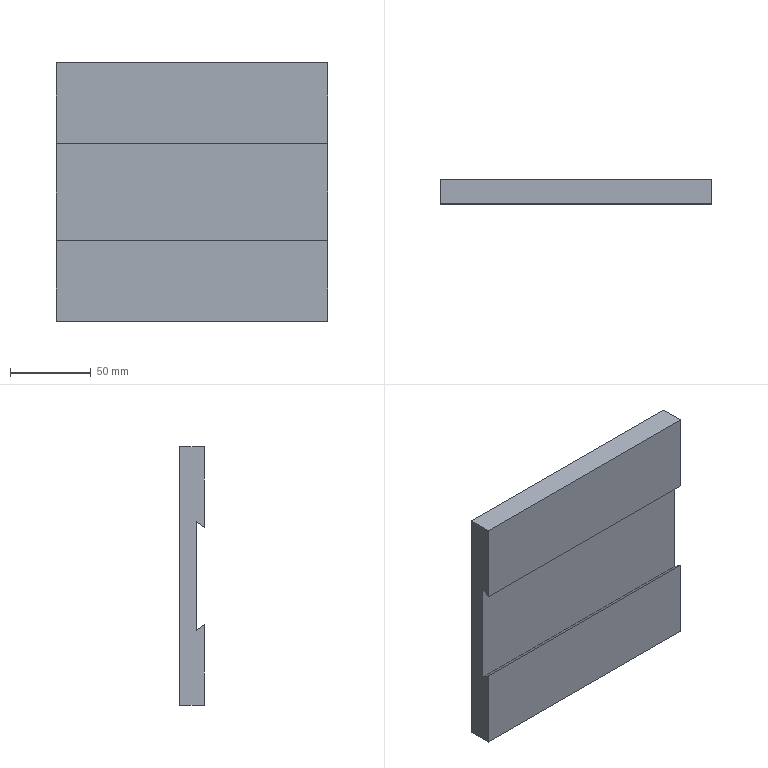Part | STEP file | 03-26 Tray support slide plate | 1 solid | 10 faces | box 168 x 15 x 160 mm | volume 349859 mm3 | plane 10
STEP:
#1=CARTESIAN_POINT('',(0.,0.,0.));
#2=DIRECTION('',(0.,0.,1.));
#3=DIRECTION('',(1.,0.,0.));
#4=AXIS2_PLACEMENT_3D('',#1,#2,#3);
#5=CARTESIAN_POINT('',(-168.,15.,80.));
#6=VERTEX_POINT('',#5);
#7=CARTESIAN_POINT('',(-168.,0.,80.));
#8=VERTEX_POINT('',#7);
#9=CARTESIAN_POINT('',(-168.,7.5,80.));
#10=DIRECTION('',(0.,-1.,0.));
#11=VECTOR('',#10,1.);
#12=LINE('',#9,#11);
#13=CARTESIAN_POINT('',(-168.,0.,80.));
#14=DIRECTION('',(0.,0.,1.));
#15=DIRECTION('',(1.,0.,0.));
#16=AXIS2_PLACEMENT_3D('',#13,#14,#15);
#17=PLANE('',#16);
#18=CARTESIAN_POINT('',(0.,7.5));
#19=DIRECTION('',(0.,-1.));
#20=VECTOR('',#19,1.);
#21=LINE('',#18,#20);
#22=(GEOMETRIC_REPRESENTATION_CONTEXT(2)PARAMETRIC_REPRESENTATION_CONTEXT()REPRESENTATION_CONTEXT('',''));
#23=DEFINITIONAL_REPRESENTATION('',(#21),#22);
#24=PCURVE('',#17,#23);
#25=CARTESIAN_POINT('',(-168.,0.,80.));
#26=DIRECTION('',(1.,0.,0.));
#27=DIRECTION('',(0.,0.,-1.));
#28=AXIS2_PLACEMENT_3D('',#25,#26,#27);
#29=PLANE('',#28);
#30=CARTESIAN_POINT('',(0.,7.5));
#31=DIRECTION('',(0.,-1.));
#32=VECTOR('',#31,1.);
#33=LINE('',#30,#32);
#34=(GEOMETRIC_REPRESENTATION_CONTEXT(2)PARAMETRIC_REPRESENTATION_CONTEXT()REPRESENTATION_CONTEXT('',''));
#35=DEFINITIONAL_REPRESENTATION('',(#33),#34);
#36=PCURVE('',#29,#35);
#37=SURFACE_CURVE('',#12,(#24,#36),.PCURVE_S1.);
#38=EDGE_CURVE('',#6,#8,#37,.T.);
#39=ORIENTED_EDGE('',*,*,#38,.T.);
#40=CARTESIAN_POINT('',(0.,0.,80.));
#41=VERTEX_POINT('',#40);
#42=CARTESIAN_POINT('',(-84.,0.,80.));
#43=DIRECTION('',(1.,0.,0.));
#44=VECTOR('',#43,1.);
#45=LINE('',#42,#44);
#46=CARTESIAN_POINT('',(84.,0.));
#47=DIRECTION('',(1.,0.));
#48=VECTOR('',#47,1.);
#49=LINE('',#46,#48);
#50=(GEOMETRIC_REPRESENTATION_CONTEXT(2)PARAMETRIC_REPRESENTATION_CONTEXT()REPRESENTATION_CONTEXT('',''));
#51=DEFINITIONAL_REPRESENTATION('',(#49),#50);
#52=PCURVE('',#17,#51);
#53=CARTESIAN_POINT('',(-168.,0.,80.));
#54=DIRECTION('',(0.,-1.,0.));
#55=DIRECTION('',(0.,0.,-1.));
#56=AXIS2_PLACEMENT_3D('',#53,#54,#55);
#57=PLANE('',#56);
#58=CARTESIAN_POINT('',(0.,84.));
#59=DIRECTION('',(0.,1.));
#60=VECTOR('',#59,1.);
#61=LINE('',#58,#60);
#62=(GEOMETRIC_REPRESENTATION_CONTEXT(2)PARAMETRIC_REPRESENTATION_CONTEXT()REPRESENTATION_CONTEXT('',''));
#63=DEFINITIONAL_REPRESENTATION('',(#61),#62);
#64=PCURVE('',#57,#63);
#65=SURFACE_CURVE('',#45,(#52,#64),.PCURVE_S1.);
#66=EDGE_CURVE('',#8,#41,#65,.T.);
#67=ORIENTED_EDGE('',*,*,#66,.T.);
#68=CARTESIAN_POINT('',(0.,15.,80.));
#69=VERTEX_POINT('',#68);
#70=CARTESIAN_POINT('',(0.,7.5,80.));
#71=DIRECTION('',(0.,1.,0.));
#72=VECTOR('',#71,1.);
#73=LINE('',#70,#72);
#74=CARTESIAN_POINT('',(168.,7.5));
#75=DIRECTION('',(0.,1.));
#76=VECTOR('',#75,1.);
#77=LINE('',#74,#76);
#78=(GEOMETRIC_REPRESENTATION_CONTEXT(2)PARAMETRIC_REPRESENTATION_CONTEXT()REPRESENTATION_CONTEXT('',''));
#79=DEFINITIONAL_REPRESENTATION('',(#77),#78);
#80=PCURVE('',#17,#79);
#81=CARTESIAN_POINT('',(0.,0.,80.));
#82=DIRECTION('',(1.,0.,0.));
#83=DIRECTION('',(0.,0.,-1.));
#84=AXIS2_PLACEMENT_3D('',#81,#82,#83);
#85=PLANE('',#84);
#86=CARTESIAN_POINT('',(0.,7.5));
#87=DIRECTION('',(0.,1.));
#88=VECTOR('',#87,1.);
#89=LINE('',#86,#88);
#90=(GEOMETRIC_REPRESENTATION_CONTEXT(2)PARAMETRIC_REPRESENTATION_CONTEXT()REPRESENTATION_CONTEXT('',''));
#91=DEFINITIONAL_REPRESENTATION('',(#89),#90);
#92=PCURVE('',#85,#91);
#93=SURFACE_CURVE('',#73,(#80,#92),.PCURVE_S1.);
#94=EDGE_CURVE('',#41,#69,#93,.T.);
#95=ORIENTED_EDGE('',*,*,#94,.T.);
#96=CARTESIAN_POINT('',(-84.,15.,80.));
#97=DIRECTION('',(-1.,0.,0.));
#98=VECTOR('',#97,1.);
#99=LINE('',#96,#98);
#100=CARTESIAN_POINT('',(84.,15.));
#101=DIRECTION('',(-1.,0.));
#102=VECTOR('',#101,1.);
#103=LINE('',#100,#102);
#104=(GEOMETRIC_REPRESENTATION_CONTEXT(2)PARAMETRIC_REPRESENTATION_CONTEXT()REPRESENTATION_CONTEXT('',''));
#105=DEFINITIONAL_REPRESENTATION('',(#103),#104);
#106=PCURVE('',#17,#105);
#107=CARTESIAN_POINT('',(-168.,15.,-80.));
#108=DIRECTION('',(0.,1.,0.));
#109=DIRECTION('',(0.,0.,1.));
#110=AXIS2_PLACEMENT_3D('',#107,#108,#109);
#111=PLANE('',#110);
#112=CARTESIAN_POINT('',(160.,84.));
#113=DIRECTION('',(0.,-1.));
#114=VECTOR('',#113,1.);
#115=LINE('',#112,#114);
#116=(GEOMETRIC_REPRESENTATION_CONTEXT(2)PARAMETRIC_REPRESENTATION_CONTEXT()REPRESENTATION_CONTEXT('',''));
#117=DEFINITIONAL_REPRESENTATION('',(#115),#116);
#118=PCURVE('',#111,#117);
#119=SURFACE_CURVE('',#99,(#106,#118),.PCURVE_S1.);
#120=EDGE_CURVE('',#69,#6,#119,.T.);
#121=ORIENTED_EDGE('',*,*,#120,.T.);
#122=EDGE_LOOP('',(#39,#67,#95,#121));
#123=FACE_BOUND('',#122,.T.);
#124=ADVANCED_FACE('',(#123),#17,.T.);
#125=CARTESIAN_POINT('',(-168.,0.,30.));
#126=VERTEX_POINT('',#125);
#127=CARTESIAN_POINT('',(-168.,0.,55.));
#128=DIRECTION('',(0.,0.,-1.));
#129=VECTOR('',#128,1.);
#130=LINE('',#127,#129);
#131=CARTESIAN_POINT('',(25.,0.));
#132=DIRECTION('',(1.,0.));
#133=VECTOR('',#132,1.);
#134=LINE('',#131,#133);
#135=(GEOMETRIC_REPRESENTATION_CONTEXT(2)PARAMETRIC_REPRESENTATION_CONTEXT()REPRESENTATION_CONTEXT('',''));
#136=DEFINITIONAL_REPRESENTATION('',(#134),#135);
#137=PCURVE('',#57,#136);
#138=CARTESIAN_POINT('',(25.,0.));
#139=DIRECTION('',(1.,0.));
#140=VECTOR('',#139,1.);
#141=LINE('',#138,#140);
#142=(GEOMETRIC_REPRESENTATION_CONTEXT(2)PARAMETRIC_REPRESENTATION_CONTEXT()REPRESENTATION_CONTEXT('',''));
#143=DEFINITIONAL_REPRESENTATION('',(#141),#142);
#144=PCURVE('',#29,#143);
#145=SURFACE_CURVE('',#130,(#137,#144),.PCURVE_S1.);
#146=EDGE_CURVE('',#8,#126,#145,.T.);
#147=ORIENTED_EDGE('',*,*,#146,.T.);
#148=CARTESIAN_POINT('',(0.,0.,30.));
#149=VERTEX_POINT('',#148);
#150=CARTESIAN_POINT('',(-84.,0.,30.));
#151=DIRECTION('',(1.,0.,0.));
#152=VECTOR('',#151,1.);
#153=LINE('',#150,#152);
#154=CARTESIAN_POINT('',(50.,84.));
#155=DIRECTION('',(0.,1.));
#156=VECTOR('',#155,1.);
#157=LINE('',#154,#156);
#158=(GEOMETRIC_REPRESENTATION_CONTEXT(2)PARAMETRIC_REPRESENTATION_CONTEXT()REPRESENTATION_CONTEXT('',''));
#159=DEFINITIONAL_REPRESENTATION('',(#157),#158);
#160=PCURVE('',#57,#159);
#161=CARTESIAN_POINT('',(-168.,0.,30.));
#162=DIRECTION('',(0.,0.5736,-0.8192));
#163=DIRECTION('',(0.,0.8192,0.5736));
#164=AXIS2_PLACEMENT_3D('',#161,#162,#163);
#165=PLANE('',#164);
#166=CARTESIAN_POINT('',(0.,84.));
#167=DIRECTION('',(0.,1.));
#168=VECTOR('',#167,1.);
#169=LINE('',#166,#168);
#170=(GEOMETRIC_REPRESENTATION_CONTEXT(2)PARAMETRIC_REPRESENTATION_CONTEXT()REPRESENTATION_CONTEXT('',''));
#171=DEFINITIONAL_REPRESENTATION('',(#169),#170);
#172=PCURVE('',#165,#171);
#173=SURFACE_CURVE('',#153,(#160,#172),.PCURVE_S1.);
#174=EDGE_CURVE('',#126,#149,#173,.T.);
#175=ORIENTED_EDGE('',*,*,#174,.T.);
#176=CARTESIAN_POINT('',(0.,0.,55.));
#177=DIRECTION('',(0.,0.,1.));
#178=VECTOR('',#177,1.);
#179=LINE('',#176,#178);
#180=CARTESIAN_POINT('',(25.,168.));
#181=DIRECTION('',(-1.,0.));
#182=VECTOR('',#181,1.);
#183=LINE('',#180,#182);
#184=(GEOMETRIC_REPRESENTATION_CONTEXT(2)PARAMETRIC_REPRESENTATION_CONTEXT()REPRESENTATION_CONTEXT('',''));
#185=DEFINITIONAL_REPRESENTATION('',(#183),#184);
#186=PCURVE('',#57,#185);
#187=CARTESIAN_POINT('',(25.,0.));
#188=DIRECTION('',(-1.,0.));
#189=VECTOR('',#188,1.);
#190=LINE('',#187,#189);
#191=(GEOMETRIC_REPRESENTATION_CONTEXT(2)PARAMETRIC_REPRESENTATION_CONTEXT()REPRESENTATION_CONTEXT('',''));
#192=DEFINITIONAL_REPRESENTATION('',(#190),#191);
#193=PCURVE('',#85,#192);
#194=SURFACE_CURVE('',#179,(#186,#193),.PCURVE_S1.);
#195=EDGE_CURVE('',#149,#41,#194,.T.);
#196=ORIENTED_EDGE('',*,*,#195,.T.);
#197=ORIENTED_EDGE('',*,*,#66,.F.);
#198=EDGE_LOOP('',(#147,#175,#196,#197));
#199=FACE_BOUND('',#198,.T.);
#200=ADVANCED_FACE('',(#199),#57,.T.);
#201=CARTESIAN_POINT('',(-168.,15.,-80.));
#202=VERTEX_POINT('',#201);
#203=CARTESIAN_POINT('',(-168.,15.,0.));
#204=DIRECTION('',(0.,0.,1.));
#205=VECTOR('',#204,1.);
#206=LINE('',#203,#205);
#207=CARTESIAN_POINT('',(80.,15.));
#208=DIRECTION('',(-1.,0.));
#209=VECTOR('',#208,1.);
#210=LINE('',#207,#209);
#211=(GEOMETRIC_REPRESENTATION_CONTEXT(2)PARAMETRIC_REPRESENTATION_CONTEXT()REPRESENTATION_CONTEXT('',''));
#212=DEFINITIONAL_REPRESENTATION('',(#210),#211);
#213=PCURVE('',#29,#212);
#214=CARTESIAN_POINT('',(80.,0.));
#215=DIRECTION('',(1.,0.));
#216=VECTOR('',#215,1.);
#217=LINE('',#214,#216);
#218=(GEOMETRIC_REPRESENTATION_CONTEXT(2)PARAMETRIC_REPRESENTATION_CONTEXT()REPRESENTATION_CONTEXT('',''));
#219=DEFINITIONAL_REPRESENTATION('',(#217),#218);
#220=PCURVE('',#111,#219);
#221=SURFACE_CURVE('',#206,(#213,#220),.PCURVE_S1.);
#222=EDGE_CURVE('',#202,#6,#221,.T.);
#223=ORIENTED_EDGE('',*,*,#222,.F.);
#224=CARTESIAN_POINT('',(-168.,0.,-80.));
#225=VERTEX_POINT('',#224);
#226=CARTESIAN_POINT('',(-168.,7.5,-80.));
#227=DIRECTION('',(0.,1.,0.));
#228=VECTOR('',#227,1.);
#229=LINE('',#226,#228);
#230=CARTESIAN_POINT('',(160.,7.5));
#231=DIRECTION('',(0.,1.));
#232=VECTOR('',#231,1.);
#233=LINE('',#230,#232);
#234=(GEOMETRIC_REPRESENTATION_CONTEXT(2)PARAMETRIC_REPRESENTATION_CONTEXT()REPRESENTATION_CONTEXT('',''));
#235=DEFINITIONAL_REPRESENTATION('',(#233),#234);
#236=PCURVE('',#29,#235);
#237=CARTESIAN_POINT('',(0.,0.,-80.));
#238=DIRECTION('',(0.,0.,-1.));
#239=DIRECTION('',(-1.,0.,0.));
#240=AXIS2_PLACEMENT_3D('',#237,#238,#239);
#241=PLANE('',#240);
#242=CARTESIAN_POINT('',(168.,7.5));
#243=DIRECTION('',(0.,1.));
#244=VECTOR('',#243,1.);
#245=LINE('',#242,#244);
#246=(GEOMETRIC_REPRESENTATION_CONTEXT(2)PARAMETRIC_REPRESENTATION_CONTEXT()REPRESENTATION_CONTEXT('',''));
#247=DEFINITIONAL_REPRESENTATION('',(#245),#246);
#248=PCURVE('',#241,#247);
#249=SURFACE_CURVE('',#229,(#236,#248),.PCURVE_S1.);
#250=EDGE_CURVE('',#225,#202,#249,.T.);
#251=ORIENTED_EDGE('',*,*,#250,.F.);
#252=CARTESIAN_POINT('',(-168.,0.,-30.));
#253=VERTEX_POINT('',#252);
#254=CARTESIAN_POINT('',(-168.,0.,0.));
#255=DIRECTION('',(0.,0.,-1.));
#256=VECTOR('',#255,1.);
#257=LINE('',#254,#256);
#258=CARTESIAN_POINT('',(80.,0.));
#259=DIRECTION('',(1.,0.));
#260=VECTOR('',#259,1.);
#261=LINE('',#258,#260);
#262=(GEOMETRIC_REPRESENTATION_CONTEXT(2)PARAMETRIC_REPRESENTATION_CONTEXT()REPRESENTATION_CONTEXT('',''));
#263=DEFINITIONAL_REPRESENTATION('',(#261),#262);
#264=PCURVE('',#29,#263);
#265=CARTESIAN_POINT('',(-168.,0.,-30.));
#266=DIRECTION('',(0.,-1.,0.));
#267=DIRECTION('',(0.,0.,-1.));
#268=AXIS2_PLACEMENT_3D('',#265,#266,#267);
#269=PLANE('',#268);
#270=CARTESIAN_POINT('',(-30.,0.));
#271=DIRECTION('',(1.,0.));
#272=VECTOR('',#271,1.);
#273=LINE('',#270,#272);
#274=(GEOMETRIC_REPRESENTATION_CONTEXT(2)PARAMETRIC_REPRESENTATION_CONTEXT()REPRESENTATION_CONTEXT('',''));
#275=DEFINITIONAL_REPRESENTATION('',(#273),#274);
#276=PCURVE('',#269,#275);
#277=SURFACE_CURVE('',#257,(#264,#276),.PCURVE_S1.);
#278=EDGE_CURVE('',#253,#225,#277,.T.);
#279=ORIENTED_EDGE('',*,*,#278,.F.);
#280=CARTESIAN_POINT('',(-168.,5.,-33.501));
#281=VERTEX_POINT('',#280);
#282=CARTESIAN_POINT('',(-168.,5.,-33.501));
#283=DIRECTION('',(0.,-0.8192,0.5736));
#284=VECTOR('',#283,1.);
#285=LINE('',#282,#284);
#286=CARTESIAN_POINT('',(113.501,5.));
#287=DIRECTION('',(-0.5736,-0.8192));
#288=VECTOR('',#287,1.);
#289=LINE('',#286,#288);
#290=(GEOMETRIC_REPRESENTATION_CONTEXT(2)PARAMETRIC_REPRESENTATION_CONTEXT()REPRESENTATION_CONTEXT('',''));
#291=DEFINITIONAL_REPRESENTATION('',(#289),#290);
#292=PCURVE('',#29,#291);
#293=CARTESIAN_POINT('',(-168.,5.,-33.501));
#294=DIRECTION('',(0.,0.5736,0.8192));
#295=DIRECTION('',(0.,-0.8192,0.5736));
#296=AXIS2_PLACEMENT_3D('',#293,#294,#295);
#297=PLANE('',#296);
#298=CARTESIAN_POINT('',(0.,0.));
#299=DIRECTION('',(1.,0.));
#300=VECTOR('',#299,1.);
#301=LINE('',#298,#300);
#302=(GEOMETRIC_REPRESENTATION_CONTEXT(2)PARAMETRIC_REPRESENTATION_CONTEXT()REPRESENTATION_CONTEXT('',''));
#303=DEFINITIONAL_REPRESENTATION('',(#301),#302);
#304=PCURVE('',#297,#303);
#305=SURFACE_CURVE('',#285,(#292,#304),.PCURVE_S1.);
#306=EDGE_CURVE('',#281,#253,#305,.T.);
#307=ORIENTED_EDGE('',*,*,#306,.F.);
#308=CARTESIAN_POINT('',(-168.,5.,33.501));
#309=VERTEX_POINT('',#308);
#310=CARTESIAN_POINT('',(-168.,5.,0.));
#311=DIRECTION('',(0.,0.,-1.));
#312=VECTOR('',#311,1.);
#313=LINE('',#310,#312);
#314=CARTESIAN_POINT('',(80.,5.));
#315=DIRECTION('',(1.,0.));
#316=VECTOR('',#315,1.);
#317=LINE('',#314,#316);
#318=(GEOMETRIC_REPRESENTATION_CONTEXT(2)PARAMETRIC_REPRESENTATION_CONTEXT()REPRESENTATION_CONTEXT('',''));
#319=DEFINITIONAL_REPRESENTATION('',(#317),#318);
#320=PCURVE('',#29,#319);
#321=CARTESIAN_POINT('',(-168.,5.,33.501));
#322=DIRECTION('',(0.,-1.,0.));
#323=DIRECTION('',(0.,0.,-1.));
#324=AXIS2_PLACEMENT_3D('',#321,#322,#323);
#325=PLANE('',#324);
#326=CARTESIAN_POINT('',(33.501,0.));
#327=DIRECTION('',(1.,0.));
#328=VECTOR('',#327,1.);
#329=LINE('',#326,#328);
#330=(GEOMETRIC_REPRESENTATION_CONTEXT(2)PARAMETRIC_REPRESENTATION_CONTEXT()REPRESENTATION_CONTEXT('',''));
#331=DEFINITIONAL_REPRESENTATION('',(#329),#330);
#332=PCURVE('',#325,#331);
#333=SURFACE_CURVE('',#313,(#320,#332),.PCURVE_S1.);
#334=EDGE_CURVE('',#309,#281,#333,.T.);
#335=ORIENTED_EDGE('',*,*,#334,.F.);
#336=CARTESIAN_POINT('',(-168.,0.,30.));
#337=DIRECTION('',(0.,0.8192,0.5736));
#338=VECTOR('',#337,1.);
#339=LINE('',#336,#338);
#340=CARTESIAN_POINT('',(50.,0.));
#341=DIRECTION('',(-0.5736,0.8192));
#342=VECTOR('',#341,1.);
#343=LINE('',#340,#342);
#344=(GEOMETRIC_REPRESENTATION_CONTEXT(2)PARAMETRIC_REPRESENTATION_CONTEXT()REPRESENTATION_CONTEXT('',''));
#345=DEFINITIONAL_REPRESENTATION('',(#343),#344);
#346=PCURVE('',#29,#345);
#347=CARTESIAN_POINT('',(0.,0.));
#348=DIRECTION('',(1.,0.));
#349=VECTOR('',#348,1.);
#350=LINE('',#347,#349);
#351=(GEOMETRIC_REPRESENTATION_CONTEXT(2)PARAMETRIC_REPRESENTATION_CONTEXT()REPRESENTATION_CONTEXT('',''));
#352=DEFINITIONAL_REPRESENTATION('',(#350),#351);
#353=PCURVE('',#165,#352);
#354=SURFACE_CURVE('',#339,(#346,#353),.PCURVE_S1.);
#355=EDGE_CURVE('',#126,#309,#354,.T.);
#356=ORIENTED_EDGE('',*,*,#355,.F.);
#357=ORIENTED_EDGE('',*,*,#146,.F.);
#358=ORIENTED_EDGE('',*,*,#38,.F.);
#359=EDGE_LOOP('',(#223,#251,#279,#307,#335,#356,#357,#358));
#360=FACE_BOUND('',#359,.T.);
#361=ADVANCED_FACE('',(#360),#29,.F.);
#362=ORIENTED_EDGE('',*,*,#222,.T.);
#363=ORIENTED_EDGE('',*,*,#120,.F.);
#364=CARTESIAN_POINT('',(0.,15.,-80.));
#365=VERTEX_POINT('',#364);
#366=CARTESIAN_POINT('',(0.,15.,0.));
#367=DIRECTION('',(0.,0.,-1.));
#368=VECTOR('',#367,1.);
#369=LINE('',#366,#368);
#370=CARTESIAN_POINT('',(80.,168.));
#371=DIRECTION('',(-1.,0.));
#372=VECTOR('',#371,1.);
#373=LINE('',#370,#372);
#374=(GEOMETRIC_REPRESENTATION_CONTEXT(2)PARAMETRIC_REPRESENTATION_CONTEXT()REPRESENTATION_CONTEXT('',''));
#375=DEFINITIONAL_REPRESENTATION('',(#373),#374);
#376=PCURVE('',#111,#375);
#377=CARTESIAN_POINT('',(80.,15.));
#378=DIRECTION('',(1.,0.));
#379=VECTOR('',#378,1.);
#380=LINE('',#377,#379);
#381=(GEOMETRIC_REPRESENTATION_CONTEXT(2)PARAMETRIC_REPRESENTATION_CONTEXT()REPRESENTATION_CONTEXT('',''));
#382=DEFINITIONAL_REPRESENTATION('',(#380),#381);
#383=PCURVE('',#85,#382);
#384=SURFACE_CURVE('',#369,(#376,#383),.PCURVE_S1.);
#385=EDGE_CURVE('',#69,#365,#384,.T.);
#386=ORIENTED_EDGE('',*,*,#385,.T.);
#387=CARTESIAN_POINT('',(-84.,15.,-80.));
#388=DIRECTION('',(-1.,0.,0.));
#389=VECTOR('',#388,1.);
#390=LINE('',#387,#389);
#391=CARTESIAN_POINT('',(0.,84.));
#392=DIRECTION('',(0.,-1.));
#393=VECTOR('',#392,1.);
#394=LINE('',#391,#393);
#395=(GEOMETRIC_REPRESENTATION_CONTEXT(2)PARAMETRIC_REPRESENTATION_CONTEXT()REPRESENTATION_CONTEXT('',''));
#396=DEFINITIONAL_REPRESENTATION('',(#394),#395);
#397=PCURVE('',#111,#396);
#398=CARTESIAN_POINT('',(84.,15.));
#399=DIRECTION('',(1.,0.));
#400=VECTOR('',#399,1.);
#401=LINE('',#398,#400);
#402=(GEOMETRIC_REPRESENTATION_CONTEXT(2)PARAMETRIC_REPRESENTATION_CONTEXT()REPRESENTATION_CONTEXT('',''));
#403=DEFINITIONAL_REPRESENTATION('',(#401),#402);
#404=PCURVE('',#241,#403);
#405=SURFACE_CURVE('',#390,(#397,#404),.PCURVE_S1.);
#406=EDGE_CURVE('',#365,#202,#405,.T.);
#407=ORIENTED_EDGE('',*,*,#406,.T.);
#408=EDGE_LOOP('',(#362,#363,#386,#407));
#409=FACE_BOUND('',#408,.T.);
#410=ADVANCED_FACE('',(#409),#111,.T.);
#411=CARTESIAN_POINT('',(0.,0.,-80.));
#412=VERTEX_POINT('',#411);
#413=CARTESIAN_POINT('',(0.,7.5,-80.));
#414=DIRECTION('',(0.,1.,0.));
#415=VECTOR('',#414,1.);
#416=LINE('',#413,#415);
#417=CARTESIAN_POINT('',(160.,7.5));
#418=DIRECTION('',(0.,1.));
#419=VECTOR('',#418,1.);
#420=LINE('',#417,#419);
#421=(GEOMETRIC_REPRESENTATION_CONTEXT(2)PARAMETRIC_REPRESENTATION_CONTEXT()REPRESENTATION_CONTEXT('',''));
#422=DEFINITIONAL_REPRESENTATION('',(#420),#421);
#423=PCURVE('',#85,#422);
#424=CARTESIAN_POINT('',(0.,7.5));
#425=DIRECTION('',(0.,1.));
#426=VECTOR('',#425,1.);
#427=LINE('',#424,#426);
#428=(GEOMETRIC_REPRESENTATION_CONTEXT(2)PARAMETRIC_REPRESENTATION_CONTEXT()REPRESENTATION_CONTEXT('',''));
#429=DEFINITIONAL_REPRESENTATION('',(#427),#428);
#430=PCURVE('',#241,#429);
#431=SURFACE_CURVE('',#416,(#423,#430),.PCURVE_S1.);
#432=EDGE_CURVE('',#412,#365,#431,.T.);
#433=ORIENTED_EDGE('',*,*,#432,.T.);
#434=ORIENTED_EDGE('',*,*,#385,.F.);
#435=ORIENTED_EDGE('',*,*,#94,.F.);
#436=ORIENTED_EDGE('',*,*,#195,.F.);
#437=CARTESIAN_POINT('',(0.,5.,33.501));
#438=VERTEX_POINT('',#437);
#439=CARTESIAN_POINT('',(0.,0.,30.));
#440=DIRECTION('',(0.,0.8192,0.5736));
#441=VECTOR('',#440,1.);
#442=LINE('',#439,#441);
#443=CARTESIAN_POINT('',(50.,0.));
#444=DIRECTION('',(-0.5736,0.8192));
#445=VECTOR('',#444,1.);
#446=LINE('',#443,#445);
#447=(GEOMETRIC_REPRESENTATION_CONTEXT(2)PARAMETRIC_REPRESENTATION_CONTEXT()REPRESENTATION_CONTEXT('',''));
#448=DEFINITIONAL_REPRESENTATION('',(#446),#447);
#449=PCURVE('',#85,#448);
#450=CARTESIAN_POINT('',(0.,168.));
#451=DIRECTION('',(1.,0.));
#452=VECTOR('',#451,1.);
#453=LINE('',#450,#452);
#454=(GEOMETRIC_REPRESENTATION_CONTEXT(2)PARAMETRIC_REPRESENTATION_CONTEXT()REPRESENTATION_CONTEXT('',''));
#455=DEFINITIONAL_REPRESENTATION('',(#453),#454);
#456=PCURVE('',#165,#455);
#457=SURFACE_CURVE('',#442,(#449,#456),.PCURVE_S1.);
#458=EDGE_CURVE('',#149,#438,#457,.T.);
#459=ORIENTED_EDGE('',*,*,#458,.T.);
#460=CARTESIAN_POINT('',(0.,5.,-33.501));
#461=VERTEX_POINT('',#460);
#462=CARTESIAN_POINT('',(0.,5.,0.));
#463=DIRECTION('',(0.,0.,-1.));
#464=VECTOR('',#463,1.);
#465=LINE('',#462,#464);
#466=CARTESIAN_POINT('',(80.,5.));
#467=DIRECTION('',(1.,0.));
#468=VECTOR('',#467,1.);
#469=LINE('',#466,#468);
#470=(GEOMETRIC_REPRESENTATION_CONTEXT(2)PARAMETRIC_REPRESENTATION_CONTEXT()REPRESENTATION_CONTEXT('',''));
#471=DEFINITIONAL_REPRESENTATION('',(#469),#470);
#472=PCURVE('',#85,#471);
#473=CARTESIAN_POINT('',(33.501,168.));
#474=DIRECTION('',(1.,0.));
#475=VECTOR('',#474,1.);
#476=LINE('',#473,#475);
#477=(GEOMETRIC_REPRESENTATION_CONTEXT(2)PARAMETRIC_REPRESENTATION_CONTEXT()REPRESENTATION_CONTEXT('',''));
#478=DEFINITIONAL_REPRESENTATION('',(#476),#477);
#479=PCURVE('',#325,#478);
#480=SURFACE_CURVE('',#465,(#472,#479),.PCURVE_S1.);
#481=EDGE_CURVE('',#438,#461,#480,.T.);
#482=ORIENTED_EDGE('',*,*,#481,.T.);
#483=CARTESIAN_POINT('',(0.,0.,-30.));
#484=VERTEX_POINT('',#483);
#485=CARTESIAN_POINT('',(0.,5.,-33.501));
#486=DIRECTION('',(0.,-0.8192,0.5736));
#487=VECTOR('',#486,1.);
#488=LINE('',#485,#487);
#489=CARTESIAN_POINT('',(113.501,5.));
#490=DIRECTION('',(-0.5736,-0.8192));
#491=VECTOR('',#490,1.);
#492=LINE('',#489,#491);
#493=(GEOMETRIC_REPRESENTATION_CONTEXT(2)PARAMETRIC_REPRESENTATION_CONTEXT()REPRESENTATION_CONTEXT('',''));
#494=DEFINITIONAL_REPRESENTATION('',(#492),#493);
#495=PCURVE('',#85,#494);
#496=CARTESIAN_POINT('',(-0.000000035,168.));
#497=DIRECTION('',(1.,0.));
#498=VECTOR('',#497,1.);
#499=LINE('',#496,#498);
#500=(GEOMETRIC_REPRESENTATION_CONTEXT(2)PARAMETRIC_REPRESENTATION_CONTEXT()REPRESENTATION_CONTEXT('',''));
#501=DEFINITIONAL_REPRESENTATION('',(#499),#500);
#502=PCURVE('',#297,#501);
#503=SURFACE_CURVE('',#488,(#495,#502),.PCURVE_S1.);
#504=EDGE_CURVE('',#461,#484,#503,.T.);
#505=ORIENTED_EDGE('',*,*,#504,.T.);
#506=CARTESIAN_POINT('',(0.,0.,0.));
#507=DIRECTION('',(0.,0.,-1.));
#508=VECTOR('',#507,1.);
#509=LINE('',#506,#508);
#510=CARTESIAN_POINT('',(80.,0.));
#511=DIRECTION('',(1.,0.));
#512=VECTOR('',#511,1.);
#513=LINE('',#510,#512);
#514=(GEOMETRIC_REPRESENTATION_CONTEXT(2)PARAMETRIC_REPRESENTATION_CONTEXT()REPRESENTATION_CONTEXT('',''));
#515=DEFINITIONAL_REPRESENTATION('',(#513),#514);
#516=PCURVE('',#85,#515);
#517=CARTESIAN_POINT('',(-30.,168.));
#518=DIRECTION('',(1.,0.));
#519=VECTOR('',#518,1.);
#520=LINE('',#517,#519);
#521=(GEOMETRIC_REPRESENTATION_CONTEXT(2)PARAMETRIC_REPRESENTATION_CONTEXT()REPRESENTATION_CONTEXT('',''));
#522=DEFINITIONAL_REPRESENTATION('',(#520),#521);
#523=PCURVE('',#269,#522);
#524=SURFACE_CURVE('',#509,(#516,#523),.PCURVE_S1.);
#525=EDGE_CURVE('',#484,#412,#524,.T.);
#526=ORIENTED_EDGE('',*,*,#525,.T.);
#527=EDGE_LOOP('',(#433,#434,#435,#436,#459,#482,#505,#526));
#528=FACE_BOUND('',#527,.T.);
#529=ADVANCED_FACE('',(#528),#85,.T.);
#530=ORIENTED_EDGE('',*,*,#355,.T.);
#531=CARTESIAN_POINT('',(-84.,5.,33.501));
#532=DIRECTION('',(1.,0.,0.));
#533=VECTOR('',#532,1.);
#534=LINE('',#531,#533);
#535=CARTESIAN_POINT('',(6.104,84.));
#536=DIRECTION('',(0.,1.));
#537=VECTOR('',#536,1.);
#538=LINE('',#535,#537);
#539=(GEOMETRIC_REPRESENTATION_CONTEXT(2)PARAMETRIC_REPRESENTATION_CONTEXT()REPRESENTATION_CONTEXT('',''));
#540=DEFINITIONAL_REPRESENTATION('',(#538),#539);
#541=PCURVE('',#165,#540);
#542=CARTESIAN_POINT('',(0.,84.));
#543=DIRECTION('',(0.,1.));
#544=VECTOR('',#543,1.);
#545=LINE('',#542,#544);
#546=(GEOMETRIC_REPRESENTATION_CONTEXT(2)PARAMETRIC_REPRESENTATION_CONTEXT()REPRESENTATION_CONTEXT('',''));
#547=DEFINITIONAL_REPRESENTATION('',(#545),#546);
#548=PCURVE('',#325,#547);
#549=SURFACE_CURVE('',#534,(#541,#548),.PCURVE_S1.);
#550=EDGE_CURVE('',#309,#438,#549,.T.);
#551=ORIENTED_EDGE('',*,*,#550,.T.);
#552=ORIENTED_EDGE('',*,*,#458,.F.);
#553=ORIENTED_EDGE('',*,*,#174,.F.);
#554=EDGE_LOOP('',(#530,#551,#552,#553));
#555=FACE_BOUND('',#554,.T.);
#556=ADVANCED_FACE('',(#555),#165,.T.);
#557=ORIENTED_EDGE('',*,*,#250,.T.);
#558=ORIENTED_EDGE('',*,*,#406,.F.);
#559=ORIENTED_EDGE('',*,*,#432,.F.);
#560=CARTESIAN_POINT('',(-84.,0.,-80.));
#561=DIRECTION('',(-1.,0.,0.));
#562=VECTOR('',#561,1.);
#563=LINE('',#560,#562);
#564=CARTESIAN_POINT('',(84.,0.));
#565=DIRECTION('',(1.,0.));
#566=VECTOR('',#565,1.);
#567=LINE('',#564,#566);
#568=(GEOMETRIC_REPRESENTATION_CONTEXT(2)PARAMETRIC_REPRESENTATION_CONTEXT()REPRESENTATION_CONTEXT('',''));
#569=DEFINITIONAL_REPRESENTATION('',(#567),#568);
#570=PCURVE('',#241,#569);
#571=CARTESIAN_POINT('',(50.,84.));
#572=DIRECTION('',(0.,-1.));
#573=VECTOR('',#572,1.);
#574=LINE('',#571,#573);
#575=(GEOMETRIC_REPRESENTATION_CONTEXT(2)PARAMETRIC_REPRESENTATION_CONTEXT()REPRESENTATION_CONTEXT('',''));
#576=DEFINITIONAL_REPRESENTATION('',(#574),#575);
#577=PCURVE('',#269,#576);
#578=SURFACE_CURVE('',#563,(#570,#577),.PCURVE_S1.);
#579=EDGE_CURVE('',#412,#225,#578,.T.);
#580=ORIENTED_EDGE('',*,*,#579,.T.);
#581=EDGE_LOOP('',(#557,#558,#559,#580));
#582=FACE_BOUND('',#581,.T.);
#583=ADVANCED_FACE('',(#582),#241,.T.);
#584=ORIENTED_EDGE('',*,*,#278,.T.);
#585=ORIENTED_EDGE('',*,*,#579,.F.);
#586=ORIENTED_EDGE('',*,*,#525,.F.);
#587=CARTESIAN_POINT('',(-84.,0.,-30.));
#588=DIRECTION('',(-1.,0.,0.));
#589=VECTOR('',#588,1.);
#590=LINE('',#587,#589);
#591=CARTESIAN_POINT('',(0.,84.));
#592=DIRECTION('',(0.,-1.));
#593=VECTOR('',#592,1.);
#594=LINE('',#591,#593);
#595=(GEOMETRIC_REPRESENTATION_CONTEXT(2)PARAMETRIC_REPRESENTATION_CONTEXT()REPRESENTATION_CONTEXT('',''));
#596=DEFINITIONAL_REPRESENTATION('',(#594),#595);
#597=PCURVE('',#269,#596);
#598=CARTESIAN_POINT('',(6.104,84.));
#599=DIRECTION('',(0.,-1.));
#600=VECTOR('',#599,1.);
#601=LINE('',#598,#600);
#602=(GEOMETRIC_REPRESENTATION_CONTEXT(2)PARAMETRIC_REPRESENTATION_CONTEXT()REPRESENTATION_CONTEXT('',''));
#603=DEFINITIONAL_REPRESENTATION('',(#601),#602);
#604=PCURVE('',#297,#603);
#605=SURFACE_CURVE('',#590,(#597,#604),.PCURVE_S1.);
#606=EDGE_CURVE('',#484,#253,#605,.T.);
#607=ORIENTED_EDGE('',*,*,#606,.T.);
#608=EDGE_LOOP('',(#584,#585,#586,#607));
#609=FACE_BOUND('',#608,.T.);
#610=ADVANCED_FACE('',(#609),#269,.T.);
#611=ORIENTED_EDGE('',*,*,#306,.T.);
#612=ORIENTED_EDGE('',*,*,#606,.F.);
#613=ORIENTED_EDGE('',*,*,#504,.F.);
#614=CARTESIAN_POINT('',(-84.,5.,-33.501));
#615=DIRECTION('',(-1.,0.,0.));
#616=VECTOR('',#615,1.);
#617=LINE('',#614,#616);
#618=CARTESIAN_POINT('',(0.,84.));
#619=DIRECTION('',(0.,-1.));
#620=VECTOR('',#619,1.);
#621=LINE('',#618,#620);
#622=(GEOMETRIC_REPRESENTATION_CONTEXT(2)PARAMETRIC_REPRESENTATION_CONTEXT()REPRESENTATION_CONTEXT('',''));
#623=DEFINITIONAL_REPRESENTATION('',(#621),#622);
#624=PCURVE('',#297,#623);
#625=CARTESIAN_POINT('',(67.002,84.));
#626=DIRECTION('',(0.,-1.));
#627=VECTOR('',#626,1.);
#628=LINE('',#625,#627);
#629=(GEOMETRIC_REPRESENTATION_CONTEXT(2)PARAMETRIC_REPRESENTATION_CONTEXT()REPRESENTATION_CONTEXT('',''));
#630=DEFINITIONAL_REPRESENTATION('',(#628),#629);
#631=PCURVE('',#325,#630);
#632=SURFACE_CURVE('',#617,(#624,#631),.PCURVE_S1.);
#633=EDGE_CURVE('',#461,#281,#632,.T.);
#634=ORIENTED_EDGE('',*,*,#633,.T.);
#635=EDGE_LOOP('',(#611,#612,#613,#634));
#636=FACE_BOUND('',#635,.T.);
#637=ADVANCED_FACE('',(#636),#297,.T.);
#638=ORIENTED_EDGE('',*,*,#334,.T.);
#639=ORIENTED_EDGE('',*,*,#633,.F.);
#640=ORIENTED_EDGE('',*,*,#481,.F.);
#641=ORIENTED_EDGE('',*,*,#550,.F.);
#642=EDGE_LOOP('',(#638,#639,#640,#641));
#643=FACE_BOUND('',#642,.T.);
#644=ADVANCED_FACE('',(#643),#325,.T.);
#645=CLOSED_SHELL('',(#124,#200,#361,#410,#529,#556,#583,#610,#637,#644));
#646=MANIFOLD_SOLID_BREP('',#645);
#647=(LENGTH_UNIT()NAMED_UNIT(*)SI_UNIT(.MILLI.,.METRE.));
#648=UNCERTAINTY_MEASURE_WITH_UNIT(LENGTH_MEASURE(0.0000001),#647,'','');
#649=(NAMED_UNIT(*)PLANE_ANGLE_UNIT()SI_UNIT($,.RADIAN.));
#650=(NAMED_UNIT(*)SI_UNIT($,.STERADIAN.)SOLID_ANGLE_UNIT());
#651=(GEOMETRIC_REPRESENTATION_CONTEXT(3)GLOBAL_UNCERTAINTY_ASSIGNED_CONTEXT((#648))GLOBAL_UNIT_ASSIGNED_CONTEXT((#647,#649,#650))REPRESENTATION_CONTEXT('',''));
#652=ADVANCED_BREP_SHAPE_REPRESENTATION('',(#4,#646),#651);